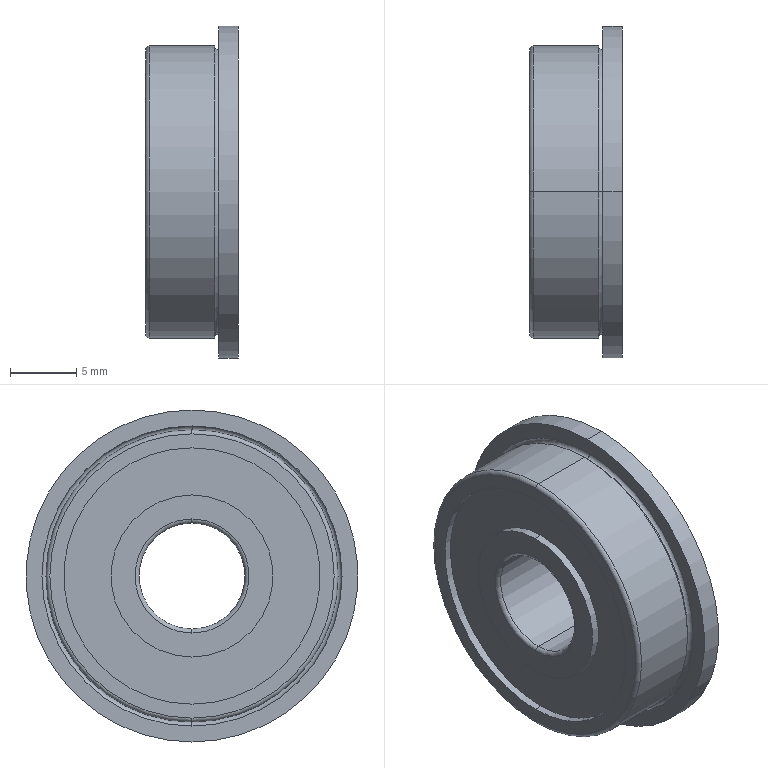Part | SolidWorks | features RefAxis 3, 3DProfileFeature 1, Revolution 1 | 1 solid | 31 faces | box 7 x 25 x 25 mm | volume 2247 mm3 | cylinder 14 | torus 10 | plane 7 | commonest cylinder face diameters 12.2 x4 19.3 x4 8 x2 22 x2 25 x2
STEP:
#1=CARTESIAN_POINT('',(5.2,0.,11.));
#2=VERTEX_POINT('',#1);
#3=CARTESIAN_POINT('',(5.5,0.,10.7));
#4=VERTEX_POINT('',#3);
#5=CARTESIAN_POINT('',(5.5,0.,11.));
#6=DIRECTION('',(0.,-1.,0.));
#7=DIRECTION('',(0.,0.,-1.));
#8=AXIS2_PLACEMENT_3D('',#5,#6,#7);
#9=CIRCLE('',#8,0.3);
#10=EDGE_CURVE('',#2,#4,#9,.T.);
#11=ORIENTED_EDGE('',*,*,#10,.T.);
#12=CARTESIAN_POINT('',(5.5,0.,-10.7));
#13=VERTEX_POINT('',#12);
#14=CARTESIAN_POINT('',(5.5,0.,0.));
#15=DIRECTION('',(-1.,0.,0.));
#16=DIRECTION('',(0.,0.,1.));
#17=AXIS2_PLACEMENT_3D('',#14,#15,#16);
#18=CIRCLE('',#17,10.7);
#19=EDGE_CURVE('',#4,#13,#18,.T.);
#20=ORIENTED_EDGE('',*,*,#19,.T.);
#21=CARTESIAN_POINT('',(5.2,0.,-11.));
#22=VERTEX_POINT('',#21);
#23=CARTESIAN_POINT('',(5.5,0.,-11.));
#24=DIRECTION('',(0.,1.,0.));
#25=DIRECTION('',(0.,0.,1.));
#26=AXIS2_PLACEMENT_3D('',#23,#24,#25);
#27=CIRCLE('',#26,0.3);
#28=EDGE_CURVE('',#22,#13,#27,.T.);
#29=ORIENTED_EDGE('',*,*,#28,.F.);
#30=CARTESIAN_POINT('',(5.2,0.,0.));
#31=DIRECTION('',(-1.,0.,0.));
#32=DIRECTION('',(0.,0.,1.));
#33=AXIS2_PLACEMENT_3D('',#30,#31,#32);
#34=CIRCLE('',#33,11.);
#35=EDGE_CURVE('',#2,#22,#34,.T.);
#36=ORIENTED_EDGE('',*,*,#35,.F.);
#37=EDGE_LOOP('',(#11,#20,#29,#36));
#38=FACE_OUTER_BOUND('',#37,.T.);
#39=CARTESIAN_POINT('',(5.5,0.,0.));
#40=DIRECTION('',(-1.,0.,0.));
#41=DIRECTION('',(0.,0.,1.));
#42=AXIS2_PLACEMENT_3D('',#39,#40,#41);
#43=TOROIDAL_SURFACE('',#42,11.,0.3);
#44=ADVANCED_FACE('',(#38),#43,.F.);
#45=ORIENTED_EDGE('',*,*,#28,.T.);
#46=CARTESIAN_POINT('',(5.5,0.,0.));
#47=DIRECTION('',(-1.,0.,0.));
#48=DIRECTION('',(0.,0.,1.));
#49=AXIS2_PLACEMENT_3D('',#46,#47,#48);
#50=CIRCLE('',#49,10.7);
#51=EDGE_CURVE('',#13,#4,#50,.T.);
#52=ORIENTED_EDGE('',*,*,#51,.T.);
#53=ORIENTED_EDGE('',*,*,#10,.F.);
#54=CARTESIAN_POINT('',(5.2,0.,0.));
#55=DIRECTION('',(-1.,0.,0.));
#56=DIRECTION('',(0.,0.,1.));
#57=AXIS2_PLACEMENT_3D('',#54,#55,#56);
#58=CIRCLE('',#57,11.);
#59=EDGE_CURVE('',#22,#2,#58,.T.);
#60=ORIENTED_EDGE('',*,*,#59,.F.);
#61=EDGE_LOOP('',(#45,#52,#53,#60));
#62=FACE_OUTER_BOUND('',#61,.T.);
#63=CARTESIAN_POINT('',(5.5,0.,0.));
#64=DIRECTION('',(-1.,0.,0.));
#65=DIRECTION('',(0.,0.,1.));
#66=AXIS2_PLACEMENT_3D('',#63,#64,#65);
#67=TOROIDAL_SURFACE('',#66,11.,0.3);
#68=ADVANCED_FACE('',(#62),#67,.F.);
#69=ORIENTED_EDGE('',*,*,#35,.T.);
#70=CARTESIAN_POINT('',(0.3,0.,-11.));
#71=VERTEX_POINT('',#70);
#72=CARTESIAN_POINT('',(22.,0.,-11.));
#73=DIRECTION('',(-1.,0.,0.));
#74=VECTOR('',#73,1000.);
#75=LINE('',#72,#74);
#76=EDGE_CURVE('',#22,#71,#75,.T.);
#77=ORIENTED_EDGE('',*,*,#76,.T.);
#78=CARTESIAN_POINT('',(0.3,0.,11.));
#79=VERTEX_POINT('',#78);
#80=CARTESIAN_POINT('',(0.3,0.,0.));
#81=DIRECTION('',(-1.,0.,0.));
#82=DIRECTION('',(0.,0.,1.));
#83=AXIS2_PLACEMENT_3D('',#80,#81,#82);
#84=CIRCLE('',#83,11.);
#85=EDGE_CURVE('',#79,#71,#84,.T.);
#86=ORIENTED_EDGE('',*,*,#85,.F.);
#87=CARTESIAN_POINT('',(22.,0.,11.));
#88=DIRECTION('',(-1.,0.,0.));
#89=VECTOR('',#88,1000.);
#90=LINE('',#87,#89);
#91=EDGE_CURVE('',#2,#79,#90,.T.);
#92=ORIENTED_EDGE('',*,*,#91,.F.);
#93=EDGE_LOOP('',(#69,#77,#86,#92));
#94=FACE_OUTER_BOUND('',#93,.T.);
#95=CARTESIAN_POINT('',(22.,0.,0.));
#96=DIRECTION('',(-1.,0.,0.));
#97=DIRECTION('',(0.,0.,1.));
#98=AXIS2_PLACEMENT_3D('',#95,#96,#97);
#99=CYLINDRICAL_SURFACE('',#98,11.);
#100=ADVANCED_FACE('',(#94),#99,.T.);
#101=ORIENTED_EDGE('',*,*,#51,.F.);
#102=CARTESIAN_POINT('',(5.5,0.,-11.3));
#103=VERTEX_POINT('',#102);
#104=CARTESIAN_POINT('',(5.5,0.,-11.));
#105=DIRECTION('',(0.,1.,0.));
#106=DIRECTION('',(0.,0.,1.));
#107=AXIS2_PLACEMENT_3D('',#104,#105,#106);
#108=CIRCLE('',#107,0.3);
#109=EDGE_CURVE('',#13,#103,#108,.T.);
#110=ORIENTED_EDGE('',*,*,#109,.T.);
#111=CARTESIAN_POINT('',(5.5,0.,11.3));
#112=VERTEX_POINT('',#111);
#113=CARTESIAN_POINT('',(5.5,0.,0.));
#114=DIRECTION('',(-1.,0.,0.));
#115=DIRECTION('',(0.,0.,1.));
#116=AXIS2_PLACEMENT_3D('',#113,#114,#115);
#117=CIRCLE('',#116,11.3);
#118=EDGE_CURVE('',#103,#112,#117,.T.);
#119=ORIENTED_EDGE('',*,*,#118,.T.);
#120=CARTESIAN_POINT('',(5.5,0.,11.));
#121=DIRECTION('',(0.,-1.,0.));
#122=DIRECTION('',(0.,0.,-1.));
#123=AXIS2_PLACEMENT_3D('',#120,#121,#122);
#124=CIRCLE('',#123,0.3);
#125=EDGE_CURVE('',#4,#112,#124,.T.);
#126=ORIENTED_EDGE('',*,*,#125,.F.);
#127=EDGE_LOOP('',(#101,#110,#119,#126));
#128=FACE_OUTER_BOUND('',#127,.T.);
#129=CARTESIAN_POINT('',(5.5,0.,0.));
#130=DIRECTION('',(-1.,0.,0.));
#131=DIRECTION('',(0.,0.,1.));
#132=AXIS2_PLACEMENT_3D('',#129,#130,#131);
#133=TOROIDAL_SURFACE('',#132,11.,0.3);
#134=ADVANCED_FACE('',(#128),#133,.F.);
#135=CARTESIAN_POINT('',(7.,0.,12.5));
#136=VERTEX_POINT('',#135);
#137=CARTESIAN_POINT('',(7.,0.,-12.5));
#138=VERTEX_POINT('',#137);
#139=CARTESIAN_POINT('',(7.,0.,0.));
#140=DIRECTION('',(-1.,0.,0.));
#141=DIRECTION('',(0.,0.,1.));
#142=AXIS2_PLACEMENT_3D('',#139,#140,#141);
#143=CIRCLE('',#142,12.5);
#144=EDGE_CURVE('',#136,#138,#143,.T.);
#145=ORIENTED_EDGE('',*,*,#144,.T.);
#146=CARTESIAN_POINT('',(5.5,0.,-12.5));
#147=VERTEX_POINT('',#146);
#148=CARTESIAN_POINT('',(22.,0.,-12.5));
#149=DIRECTION('',(-1.,0.,0.));
#150=VECTOR('',#149,1000.);
#151=LINE('',#148,#150);
#152=EDGE_CURVE('',#138,#147,#151,.T.);
#153=ORIENTED_EDGE('',*,*,#152,.T.);
#154=CARTESIAN_POINT('',(5.5,0.,12.5));
#155=VERTEX_POINT('',#154);
#156=CARTESIAN_POINT('',(5.5,0.,0.));
#157=DIRECTION('',(-1.,0.,0.));
#158=DIRECTION('',(0.,0.,1.));
#159=AXIS2_PLACEMENT_3D('',#156,#157,#158);
#160=CIRCLE('',#159,12.5);
#161=EDGE_CURVE('',#155,#147,#160,.T.);
#162=ORIENTED_EDGE('',*,*,#161,.F.);
#163=CARTESIAN_POINT('',(22.,0.,12.5));
#164=DIRECTION('',(-1.,0.,0.));
#165=VECTOR('',#164,1000.);
#166=LINE('',#163,#165);
#167=EDGE_CURVE('',#136,#155,#166,.T.);
#168=ORIENTED_EDGE('',*,*,#167,.F.);
#169=EDGE_LOOP('',(#145,#153,#162,#168));
#170=FACE_OUTER_BOUND('',#169,.T.);
#171=CARTESIAN_POINT('',(22.,0.,0.));
#172=DIRECTION('',(-1.,0.,0.));
#173=DIRECTION('',(0.,0.,1.));
#174=AXIS2_PLACEMENT_3D('',#171,#172,#173);
#175=CYLINDRICAL_SURFACE('',#174,12.5);
#176=ADVANCED_FACE('',(#170),#175,.T.);
#177=CARTESIAN_POINT('',(7.,0.,-9.65));
#178=VERTEX_POINT('',#177);
#179=CARTESIAN_POINT('',(7.,0.,9.65));
#180=VERTEX_POINT('',#179);
#181=CARTESIAN_POINT('',(7.,0.,0.));
#182=DIRECTION('',(-1.,0.,0.));
#183=DIRECTION('',(0.,0.,1.));
#184=AXIS2_PLACEMENT_3D('',#181,#182,#183);
#185=CIRCLE('',#184,9.65);
#186=EDGE_CURVE('',#178,#180,#185,.T.);
#187=ORIENTED_EDGE('',*,*,#186,.F.);
#188=CARTESIAN_POINT('',(6.4,0.,-9.65));
#189=VERTEX_POINT('',#188);
#190=CARTESIAN_POINT('',(22.,0.,-9.65));
#191=DIRECTION('',(-1.,0.,0.));
#192=VECTOR('',#191,1000.);
#193=LINE('',#190,#192);
#194=EDGE_CURVE('',#178,#189,#193,.T.);
#195=ORIENTED_EDGE('',*,*,#194,.T.);
#196=CARTESIAN_POINT('',(6.4,0.,9.65));
#197=VERTEX_POINT('',#196);
#198=CARTESIAN_POINT('',(6.4,0.,0.));
#199=DIRECTION('',(-1.,0.,0.));
#200=DIRECTION('',(0.,0.,1.));
#201=AXIS2_PLACEMENT_3D('',#198,#199,#200);
#202=CIRCLE('',#201,9.65);
#203=EDGE_CURVE('',#189,#197,#202,.T.);
#204=ORIENTED_EDGE('',*,*,#203,.T.);
#205=CARTESIAN_POINT('',(22.,0.,9.65));
#206=DIRECTION('',(-1.,0.,0.));
#207=VECTOR('',#206,1000.);
#208=LINE('',#205,#207);
#209=EDGE_CURVE('',#180,#197,#208,.T.);
#210=ORIENTED_EDGE('',*,*,#209,.F.);
#211=EDGE_LOOP('',(#187,#195,#204,#210));
#212=FACE_OUTER_BOUND('',#211,.T.);
#213=CARTESIAN_POINT('',(22.,0.,0.));
#214=DIRECTION('',(-1.,0.,0.));
#215=DIRECTION('',(0.,0.,1.));
#216=AXIS2_PLACEMENT_3D('',#213,#214,#215);
#217=CYLINDRICAL_SURFACE('',#216,9.65);
#218=ADVANCED_FACE('',(#212),#217,.F.);
#219=CARTESIAN_POINT('',(7.,0.,6.1));
#220=VERTEX_POINT('',#219);
#221=CARTESIAN_POINT('',(7.,0.,-6.1));
#222=VERTEX_POINT('',#221);
#223=CARTESIAN_POINT('',(7.,0.,0.));
#224=DIRECTION('',(-1.,0.,0.));
#225=DIRECTION('',(0.,0.,1.));
#226=AXIS2_PLACEMENT_3D('',#223,#224,#225);
#227=CIRCLE('',#226,6.1);
#228=EDGE_CURVE('',#220,#222,#227,.T.);
#229=ORIENTED_EDGE('',*,*,#228,.T.);
#230=CARTESIAN_POINT('',(6.4,0.,-6.1));
#231=VERTEX_POINT('',#230);
#232=CARTESIAN_POINT('',(22.,0.,-6.1));
#233=DIRECTION('',(-1.,0.,0.));
#234=VECTOR('',#233,1000.);
#235=LINE('',#232,#234);
#236=EDGE_CURVE('',#222,#231,#235,.T.);
#237=ORIENTED_EDGE('',*,*,#236,.T.);
#238=CARTESIAN_POINT('',(6.4,0.,6.1));
#239=VERTEX_POINT('',#238);
#240=CARTESIAN_POINT('',(6.4,0.,0.));
#241=DIRECTION('',(-1.,0.,0.));
#242=DIRECTION('',(0.,0.,1.));
#243=AXIS2_PLACEMENT_3D('',#240,#241,#242);
#244=CIRCLE('',#243,6.1);
#245=EDGE_CURVE('',#239,#231,#244,.T.);
#246=ORIENTED_EDGE('',*,*,#245,.F.);
#247=CARTESIAN_POINT('',(22.,0.,6.1));
#248=DIRECTION('',(-1.,0.,0.));
#249=VECTOR('',#248,1000.);
#250=LINE('',#247,#249);
#251=EDGE_CURVE('',#220,#239,#250,.T.);
#252=ORIENTED_EDGE('',*,*,#251,.F.);
#253=EDGE_LOOP('',(#229,#237,#246,#252));
#254=FACE_OUTER_BOUND('',#253,.T.);
#255=CARTESIAN_POINT('',(22.,0.,0.));
#256=DIRECTION('',(-1.,0.,0.));
#257=DIRECTION('',(0.,0.,1.));
#258=AXIS2_PLACEMENT_3D('',#255,#256,#257);
#259=CYLINDRICAL_SURFACE('',#258,6.1);
#260=ADVANCED_FACE('',(#254),#259,.T.);
#261=CARTESIAN_POINT('',(6.7,0.,4.));
#262=VERTEX_POINT('',#261);
#263=CARTESIAN_POINT('',(6.7,0.,-4.));
#264=VERTEX_POINT('',#263);
#265=CARTESIAN_POINT('',(6.7,0.,0.));
#266=DIRECTION('',(-1.,0.,0.));
#267=DIRECTION('',(0.,0.,1.));
#268=AXIS2_PLACEMENT_3D('',#265,#266,#267);
#269=CIRCLE('',#268,4.);
#270=EDGE_CURVE('',#262,#264,#269,.T.);
#271=ORIENTED_EDGE('',*,*,#270,.T.);
#272=CARTESIAN_POINT('',(7.,0.,-4.3));
#273=VERTEX_POINT('',#272);
#274=CARTESIAN_POINT('',(6.7,0.,-4.3));
#275=DIRECTION('',(0.,1.,0.));
#276=DIRECTION('',(0.,0.,1.));
#277=AXIS2_PLACEMENT_3D('',#274,#275,#276);
#278=CIRCLE('',#277,0.3);
#279=EDGE_CURVE('',#264,#273,#278,.T.);
#280=ORIENTED_EDGE('',*,*,#279,.T.);
#281=CARTESIAN_POINT('',(7.,0.,4.3));
#282=VERTEX_POINT('',#281);
#283=CARTESIAN_POINT('',(7.,0.,0.));
#284=DIRECTION('',(-1.,0.,0.));
#285=DIRECTION('',(0.,0.,1.));
#286=AXIS2_PLACEMENT_3D('',#283,#284,#285);
#287=CIRCLE('',#286,4.3);
#288=EDGE_CURVE('',#282,#273,#287,.T.);
#289=ORIENTED_EDGE('',*,*,#288,.F.);
#290=CARTESIAN_POINT('',(6.7,0.,4.3));
#291=DIRECTION('',(0.,-1.,0.));
#292=DIRECTION('',(0.,0.,-1.));
#293=AXIS2_PLACEMENT_3D('',#290,#291,#292);
#294=CIRCLE('',#293,0.3);
#295=EDGE_CURVE('',#262,#282,#294,.T.);
#296=ORIENTED_EDGE('',*,*,#295,.F.);
#297=EDGE_LOOP('',(#271,#280,#289,#296));
#298=FACE_OUTER_BOUND('',#297,.T.);
#299=CARTESIAN_POINT('',(6.7,0.,0.));
#300=DIRECTION('',(-1.,0.,0.));
#301=DIRECTION('',(0.,0.,1.));
#302=AXIS2_PLACEMENT_3D('',#299,#300,#301);
#303=TOROIDAL_SURFACE('',#302,4.3,0.3);
#304=ADVANCED_FACE('',(#298),#303,.T.);
#305=CARTESIAN_POINT('',(6.7,0.,0.));
#306=DIRECTION('',(-1.,0.,0.));
#307=DIRECTION('',(0.,0.,1.));
#308=AXIS2_PLACEMENT_3D('',#305,#306,#307);
#309=CIRCLE('',#308,4.);
#310=EDGE_CURVE('',#264,#262,#309,.T.);
#311=ORIENTED_EDGE('',*,*,#310,.F.);
#312=CARTESIAN_POINT('',(0.3,0.,-4.));
#313=VERTEX_POINT('',#312);
#314=CARTESIAN_POINT('',(22.,0.,-4.));
#315=DIRECTION('',(-1.,0.,0.));
#316=VECTOR('',#315,1000.);
#317=LINE('',#314,#316);
#318=EDGE_CURVE('',#264,#313,#317,.T.);
#319=ORIENTED_EDGE('',*,*,#318,.T.);
#320=CARTESIAN_POINT('',(0.3,0.,4.));
#321=VERTEX_POINT('',#320);
#322=CARTESIAN_POINT('',(0.3,0.,0.));
#323=DIRECTION('',(-1.,0.,0.));
#324=DIRECTION('',(0.,0.,1.));
#325=AXIS2_PLACEMENT_3D('',#322,#323,#324);
#326=CIRCLE('',#325,4.);
#327=EDGE_CURVE('',#313,#321,#326,.T.);
#328=ORIENTED_EDGE('',*,*,#327,.T.);
#329=CARTESIAN_POINT('',(22.,0.,4.));
#330=DIRECTION('',(-1.,0.,0.));
#331=VECTOR('',#330,1000.);
#332=LINE('',#329,#331);
#333=EDGE_CURVE('',#262,#321,#332,.T.);
#334=ORIENTED_EDGE('',*,*,#333,.F.);
#335=EDGE_LOOP('',(#311,#319,#328,#334));
#336=FACE_OUTER_BOUND('',#335,.T.);
#337=CARTESIAN_POINT('',(22.,0.,0.));
#338=DIRECTION('',(-1.,0.,0.));
#339=DIRECTION('',(0.,0.,1.));
#340=AXIS2_PLACEMENT_3D('',#337,#338,#339);
#341=CYLINDRICAL_SURFACE('',#340,4.);
#342=ADVANCED_FACE('',(#336),#341,.F.);
#343=CARTESIAN_POINT('',(0.,0.,4.3));
#344=VERTEX_POINT('',#343);
#345=CARTESIAN_POINT('',(0.,0.,-4.3));
#346=VERTEX_POINT('',#345);
#347=CARTESIAN_POINT('',(0.,0.,0.));
#348=DIRECTION('',(-1.,0.,0.));
#349=DIRECTION('',(0.,0.,1.));
#350=AXIS2_PLACEMENT_3D('',#347,#348,#349);
#351=CIRCLE('',#350,4.3);
#352=EDGE_CURVE('',#344,#346,#351,.T.);
#353=ORIENTED_EDGE('',*,*,#352,.T.);
#354=CARTESIAN_POINT('',(0.3,0.,-4.3));
#355=DIRECTION('',(0.,1.,0.));
#356=DIRECTION('',(0.,0.,1.));
#357=AXIS2_PLACEMENT_3D('',#354,#355,#356);
#358=CIRCLE('',#357,0.3);
#359=EDGE_CURVE('',#346,#313,#358,.T.);
#360=ORIENTED_EDGE('',*,*,#359,.T.);
#361=CARTESIAN_POINT('',(0.3,0.,0.));
#362=DIRECTION('',(-1.,0.,0.));
#363=DIRECTION('',(0.,0.,1.));
#364=AXIS2_PLACEMENT_3D('',#361,#362,#363);
#365=CIRCLE('',#364,4.);
#366=EDGE_CURVE('',#321,#313,#365,.T.);
#367=ORIENTED_EDGE('',*,*,#366,.F.);
#368=CARTESIAN_POINT('',(0.3,0.,4.3));
#369=DIRECTION('',(0.,-1.,0.));
#370=DIRECTION('',(0.,0.,-1.));
#371=AXIS2_PLACEMENT_3D('',#368,#369,#370);
#372=CIRCLE('',#371,0.3);
#373=EDGE_CURVE('',#344,#321,#372,.T.);
#374=ORIENTED_EDGE('',*,*,#373,.F.);
#375=EDGE_LOOP('',(#353,#360,#367,#374));
#376=FACE_OUTER_BOUND('',#375,.T.);
#377=CARTESIAN_POINT('',(0.3,0.,0.));
#378=DIRECTION('',(-1.,0.,0.));
#379=DIRECTION('',(0.,0.,1.));
#380=AXIS2_PLACEMENT_3D('',#377,#378,#379);
#381=TOROIDAL_SURFACE('',#380,4.3,0.3);
#382=ADVANCED_FACE('',(#376),#381,.T.);
#383=CARTESIAN_POINT('',(0.6,0.,6.1));
#384=VERTEX_POINT('',#383);
#385=CARTESIAN_POINT('',(0.6,0.,-6.1));
#386=VERTEX_POINT('',#385);
#387=CARTESIAN_POINT('',(0.6,0.,0.));
#388=DIRECTION('',(-1.,0.,0.));
#389=DIRECTION('',(0.,0.,1.));
#390=AXIS2_PLACEMENT_3D('',#387,#388,#389);
#391=CIRCLE('',#390,6.1);
#392=EDGE_CURVE('',#384,#386,#391,.T.);
#393=ORIENTED_EDGE('',*,*,#392,.T.);
#394=CARTESIAN_POINT('',(0.,0.,-6.1));
#395=VERTEX_POINT('',#394);
#396=CARTESIAN_POINT('',(22.,0.,-6.1));
#397=DIRECTION('',(-1.,0.,0.));
#398=VECTOR('',#397,1000.);
#399=LINE('',#396,#398);
#400=EDGE_CURVE('',#386,#395,#399,.T.);
#401=ORIENTED_EDGE('',*,*,#400,.T.);
#402=CARTESIAN_POINT('',(0.,0.,6.1));
#403=VERTEX_POINT('',#402);
#404=CARTESIAN_POINT('',(0.,0.,0.));
#405=DIRECTION('',(-1.,0.,0.));
#406=DIRECTION('',(0.,0.,1.));
#407=AXIS2_PLACEMENT_3D('',#404,#405,#406);
#408=CIRCLE('',#407,6.1);
#409=EDGE_CURVE('',#403,#395,#408,.T.);
#410=ORIENTED_EDGE('',*,*,#409,.F.);
#411=CARTESIAN_POINT('',(22.,0.,6.1));
#412=DIRECTION('',(-1.,0.,0.));
#413=VECTOR('',#412,1000.);
#414=LINE('',#411,#413);
#415=EDGE_CURVE('',#384,#403,#414,.T.);
#416=ORIENTED_EDGE('',*,*,#415,.F.);
#417=EDGE_LOOP('',(#393,#401,#410,#416));
#418=FACE_OUTER_BOUND('',#417,.T.);
#419=CARTESIAN_POINT('',(22.,0.,0.));
#420=DIRECTION('',(-1.,0.,0.));
#421=DIRECTION('',(0.,0.,1.));
#422=AXIS2_PLACEMENT_3D('',#419,#420,#421);
#423=CYLINDRICAL_SURFACE('',#422,6.1);
#424=ADVANCED_FACE('',(#418),#423,.T.);
#425=CARTESIAN_POINT('',(0.6,0.,-9.65));
#426=VERTEX_POINT('',#425);
#427=CARTESIAN_POINT('',(0.6,0.,9.65));
#428=VERTEX_POINT('',#427);
#429=CARTESIAN_POINT('',(0.6,0.,0.));
#430=DIRECTION('',(-1.,0.,0.));
#431=DIRECTION('',(0.,0.,1.));
#432=AXIS2_PLACEMENT_3D('',#429,#430,#431);
#433=CIRCLE('',#432,9.65);
#434=EDGE_CURVE('',#426,#428,#433,.T.);
#435=ORIENTED_EDGE('',*,*,#434,.F.);
#436=CARTESIAN_POINT('',(0.,0.,-9.65));
#437=VERTEX_POINT('',#436);
#438=CARTESIAN_POINT('',(22.,0.,-9.65));
#439=DIRECTION('',(-1.,0.,0.));
#440=VECTOR('',#439,1000.);
#441=LINE('',#438,#440);
#442=EDGE_CURVE('',#426,#437,#441,.T.);
#443=ORIENTED_EDGE('',*,*,#442,.T.);
#444=CARTESIAN_POINT('',(0.,0.,9.65));
#445=VERTEX_POINT('',#444);
#446=CARTESIAN_POINT('',(0.,0.,0.));
#447=DIRECTION('',(-1.,0.,0.));
#448=DIRECTION('',(0.,0.,1.));
#449=AXIS2_PLACEMENT_3D('',#446,#447,#448);
#450=CIRCLE('',#449,9.65);
#451=EDGE_CURVE('',#437,#445,#450,.T.);
#452=ORIENTED_EDGE('',*,*,#451,.T.);
#453=CARTESIAN_POINT('',(22.,0.,9.65));
#454=DIRECTION('',(-1.,0.,0.));
#455=VECTOR('',#454,1000.);
#456=LINE('',#453,#455);
#457=EDGE_CURVE('',#428,#445,#456,.T.);
#458=ORIENTED_EDGE('',*,*,#457,.F.);
#459=EDGE_LOOP('',(#435,#443,#452,#458));
#460=FACE_OUTER_BOUND('',#459,.T.);
#461=CARTESIAN_POINT('',(22.,0.,0.));
#462=DIRECTION('',(-1.,0.,0.));
#463=DIRECTION('',(0.,0.,1.));
#464=AXIS2_PLACEMENT_3D('',#461,#462,#463);
#465=CYLINDRICAL_SURFACE('',#464,9.65);
#466=ADVANCED_FACE('',(#460),#465,.F.);
#467=ORIENTED_EDGE('',*,*,#85,.T.);
#468=CARTESIAN_POINT('',(0.,0.,-10.7));
#469=VERTEX_POINT('',#468);
#470=CARTESIAN_POINT('',(0.3,0.,-10.7));
#471=DIRECTION('',(0.,1.,0.));
#472=DIRECTION('',(0.,0.,1.));
#473=AXIS2_PLACEMENT_3D('',#470,#471,#472);
#474=CIRCLE('',#473,0.3);
#475=EDGE_CURVE('',#71,#469,#474,.T.);
#476=ORIENTED_EDGE('',*,*,#475,.T.);
#477=CARTESIAN_POINT('',(0.,0.,10.7));
#478=VERTEX_POINT('',#477);
#479=CARTESIAN_POINT('',(0.,0.,0.));
#480=DIRECTION('',(-1.,0.,0.));
#481=DIRECTION('',(0.,0.,1.));
#482=AXIS2_PLACEMENT_3D('',#479,#480,#481);
#483=CIRCLE('',#482,10.7);
#484=EDGE_CURVE('',#478,#469,#483,.T.);
#485=ORIENTED_EDGE('',*,*,#484,.F.);
#486=CARTESIAN_POINT('',(0.3,0.,10.7));
#487=DIRECTION('',(0.,-1.,0.));
#488=DIRECTION('',(0.,0.,-1.));
#489=AXIS2_PLACEMENT_3D('',#486,#487,#488);
#490=CIRCLE('',#489,0.3);
#491=EDGE_CURVE('',#79,#478,#490,.T.);
#492=ORIENTED_EDGE('',*,*,#491,.F.);
#493=EDGE_LOOP('',(#467,#476,#485,#492));
#494=FACE_OUTER_BOUND('',#493,.T.);
#495=CARTESIAN_POINT('',(0.3,0.,0.));
#496=DIRECTION('',(-1.,0.,0.));
#497=DIRECTION('',(0.,0.,1.));
#498=AXIS2_PLACEMENT_3D('',#495,#496,#497);
#499=TOROIDAL_SURFACE('',#498,10.7,0.3);
#500=ADVANCED_FACE('',(#494),#499,.T.);
#501=ORIENTED_EDGE('',*,*,#475,.F.);
#502=CARTESIAN_POINT('',(0.3,0.,0.));
#503=DIRECTION('',(-1.,0.,0.));
#504=DIRECTION('',(0.,0.,1.));
#505=AXIS2_PLACEMENT_3D('',#502,#503,#504);
#506=CIRCLE('',#505,11.);
#507=EDGE_CURVE('',#71,#79,#506,.T.);
#508=ORIENTED_EDGE('',*,*,#507,.T.);
#509=ORIENTED_EDGE('',*,*,#491,.T.);
#510=CARTESIAN_POINT('',(0.,0.,0.));
#511=DIRECTION('',(-1.,0.,0.));
#512=DIRECTION('',(0.,0.,1.));
#513=AXIS2_PLACEMENT_3D('',#510,#511,#512);
#514=CIRCLE('',#513,10.7);
#515=EDGE_CURVE('',#469,#478,#514,.T.);
#516=ORIENTED_EDGE('',*,*,#515,.F.);
#517=EDGE_LOOP('',(#501,#508,#509,#516));
#518=FACE_OUTER_BOUND('',#517,.T.);
#519=CARTESIAN_POINT('',(0.3,0.,0.));
#520=DIRECTION('',(-1.,0.,0.));
#521=DIRECTION('',(0.,0.,1.));
#522=AXIS2_PLACEMENT_3D('',#519,#520,#521);
#523=TOROIDAL_SURFACE('',#522,10.7,0.3);
#524=ADVANCED_FACE('',(#518),#523,.T.);
#525=CARTESIAN_POINT('',(0.,0.,0.));
#526=DIRECTION('',(-1.,0.,0.));
#527=DIRECTION('',(0.,0.,1.));
#528=AXIS2_PLACEMENT_3D('',#525,#526,#527);
#529=CIRCLE('',#528,9.65);
#530=EDGE_CURVE('',#445,#437,#529,.T.);
#531=ORIENTED_EDGE('',*,*,#530,.F.);
#532=ORIENTED_EDGE('',*,*,#451,.F.);
#533=EDGE_LOOP('',(#531,#532));
#534=FACE_BOUND('',#533,.T.);
#535=ORIENTED_EDGE('',*,*,#484,.T.);
#536=ORIENTED_EDGE('',*,*,#515,.T.);
#537=EDGE_LOOP('',(#535,#536));
#538=FACE_OUTER_BOUND('',#537,.T.);
#539=CARTESIAN_POINT('',(0.,10.7,0.));
#540=DIRECTION('',(1.,0.,0.));
#541=DIRECTION('',(0.,0.,-1.));
#542=AXIS2_PLACEMENT_3D('',#539,#540,#541);
#543=PLANE('',#542);
#544=ADVANCED_FACE('',(#534,#538),#543,.F.);
#545=ORIENTED_EDGE('',*,*,#442,.F.);
#546=CARTESIAN_POINT('',(0.6,0.,0.));
#547=DIRECTION('',(-1.,0.,0.));
#548=DIRECTION('',(0.,0.,1.));
#549=AXIS2_PLACEMENT_3D('',#546,#547,#548);
#550=CIRCLE('',#549,9.65);
#551=EDGE_CURVE('',#428,#426,#550,.T.);
#552=ORIENTED_EDGE('',*,*,#551,.F.);
#553=ORIENTED_EDGE('',*,*,#457,.T.);
#554=ORIENTED_EDGE('',*,*,#530,.T.);
#555=EDGE_LOOP('',(#545,#552,#553,#554));
#556=FACE_OUTER_BOUND('',#555,.T.);
#557=CARTESIAN_POINT('',(22.,0.,0.));
#558=DIRECTION('',(-1.,0.,0.));
#559=DIRECTION('',(0.,0.,1.));
#560=AXIS2_PLACEMENT_3D('',#557,#558,#559);
#561=CYLINDRICAL_SURFACE('',#560,9.65);
#562=ADVANCED_FACE('',(#556),#561,.F.);
#563=ORIENTED_EDGE('',*,*,#392,.F.);
#564=CARTESIAN_POINT('',(0.6,0.,0.));
#565=DIRECTION('',(-1.,0.,0.));
#566=DIRECTION('',(0.,0.,1.));
#567=AXIS2_PLACEMENT_3D('',#564,#565,#566);
#568=CIRCLE('',#567,6.1);
#569=EDGE_CURVE('',#386,#384,#568,.T.);
#570=ORIENTED_EDGE('',*,*,#569,.F.);
#571=EDGE_LOOP('',(#563,#570));
#572=FACE_BOUND('',#571,.T.);
#573=ORIENTED_EDGE('',*,*,#551,.T.);
#574=ORIENTED_EDGE('',*,*,#434,.T.);
#575=EDGE_LOOP('',(#573,#574));
#576=FACE_OUTER_BOUND('',#575,.T.);
#577=CARTESIAN_POINT('',(0.6,9.65,0.));
#578=DIRECTION('',(1.,0.,0.));
#579=DIRECTION('',(0.,0.,-1.));
#580=AXIS2_PLACEMENT_3D('',#577,#578,#579);
#581=PLANE('',#580);
#582=ADVANCED_FACE('',(#572,#576),#581,.F.);
#583=ORIENTED_EDGE('',*,*,#400,.F.);
#584=ORIENTED_EDGE('',*,*,#569,.T.);
#585=ORIENTED_EDGE('',*,*,#415,.T.);
#586=CARTESIAN_POINT('',(0.,0.,0.));
#587=DIRECTION('',(-1.,0.,0.));
#588=DIRECTION('',(0.,0.,1.));
#589=AXIS2_PLACEMENT_3D('',#586,#587,#588);
#590=CIRCLE('',#589,6.1);
#591=EDGE_CURVE('',#395,#403,#590,.T.);
#592=ORIENTED_EDGE('',*,*,#591,.F.);
#593=EDGE_LOOP('',(#583,#584,#585,#592));
#594=FACE_OUTER_BOUND('',#593,.T.);
#595=CARTESIAN_POINT('',(22.,0.,0.));
#596=DIRECTION('',(-1.,0.,0.));
#597=DIRECTION('',(0.,0.,1.));
#598=AXIS2_PLACEMENT_3D('',#595,#596,#597);
#599=CYLINDRICAL_SURFACE('',#598,6.1);
#600=ADVANCED_FACE('',(#594),#599,.T.);
#601=ORIENTED_EDGE('',*,*,#352,.F.);
#602=CARTESIAN_POINT('',(0.,0.,0.));
#603=DIRECTION('',(-1.,0.,0.));
#604=DIRECTION('',(0.,0.,1.));
#605=AXIS2_PLACEMENT_3D('',#602,#603,#604);
#606=CIRCLE('',#605,4.3);
#607=EDGE_CURVE('',#346,#344,#606,.T.);
#608=ORIENTED_EDGE('',*,*,#607,.F.);
#609=EDGE_LOOP('',(#601,#608));
#610=FACE_BOUND('',#609,.T.);
#611=ORIENTED_EDGE('',*,*,#409,.T.);
#612=ORIENTED_EDGE('',*,*,#591,.T.);
#613=EDGE_LOOP('',(#611,#612));
#614=FACE_OUTER_BOUND('',#613,.T.);
#615=CARTESIAN_POINT('',(0.,6.1,0.));
#616=DIRECTION('',(1.,0.,0.));
#617=DIRECTION('',(0.,0.,-1.));
#618=AXIS2_PLACEMENT_3D('',#615,#616,#617);
#619=PLANE('',#618);
#620=ADVANCED_FACE('',(#610,#614),#619,.F.);
#621=ORIENTED_EDGE('',*,*,#359,.F.);
#622=ORIENTED_EDGE('',*,*,#607,.T.);
#623=ORIENTED_EDGE('',*,*,#373,.T.);
#624=ORIENTED_EDGE('',*,*,#327,.F.);
#625=EDGE_LOOP('',(#621,#622,#623,#624));
#626=FACE_OUTER_BOUND('',#625,.T.);
#627=CARTESIAN_POINT('',(0.3,0.,0.));
#628=DIRECTION('',(-1.,0.,0.));
#629=DIRECTION('',(0.,0.,1.));
#630=AXIS2_PLACEMENT_3D('',#627,#628,#629);
#631=TOROIDAL_SURFACE('',#630,4.3,0.3);
#632=ADVANCED_FACE('',(#626),#631,.T.);
#633=ORIENTED_EDGE('',*,*,#318,.F.);
#634=ORIENTED_EDGE('',*,*,#270,.F.);
#635=ORIENTED_EDGE('',*,*,#333,.T.);
#636=ORIENTED_EDGE('',*,*,#366,.T.);
#637=EDGE_LOOP('',(#633,#634,#635,#636));
#638=FACE_OUTER_BOUND('',#637,.T.);
#639=CARTESIAN_POINT('',(22.,0.,0.));
#640=DIRECTION('',(-1.,0.,0.));
#641=DIRECTION('',(0.,0.,1.));
#642=AXIS2_PLACEMENT_3D('',#639,#640,#641);
#643=CYLINDRICAL_SURFACE('',#642,4.);
#644=ADVANCED_FACE('',(#638),#643,.F.);
#645=ORIENTED_EDGE('',*,*,#279,.F.);
#646=ORIENTED_EDGE('',*,*,#310,.T.);
#647=ORIENTED_EDGE('',*,*,#295,.T.);
#648=CARTESIAN_POINT('',(7.,0.,0.));
#649=DIRECTION('',(-1.,0.,0.));
#650=DIRECTION('',(0.,0.,1.));
#651=AXIS2_PLACEMENT_3D('',#648,#649,#650);
#652=CIRCLE('',#651,4.3);
#653=EDGE_CURVE('',#273,#282,#652,.T.);
#654=ORIENTED_EDGE('',*,*,#653,.F.);
#655=EDGE_LOOP('',(#645,#646,#647,#654));
#656=FACE_OUTER_BOUND('',#655,.T.);
#657=CARTESIAN_POINT('',(6.7,0.,0.));
#658=DIRECTION('',(-1.,0.,0.));
#659=DIRECTION('',(0.,0.,1.));
#660=AXIS2_PLACEMENT_3D('',#657,#658,#659);
#661=TOROIDAL_SURFACE('',#660,4.3,0.3);
#662=ADVANCED_FACE('',(#656),#661,.T.);
#663=ORIENTED_EDGE('',*,*,#228,.F.);
#664=CARTESIAN_POINT('',(7.,0.,0.));
#665=DIRECTION('',(-1.,0.,0.));
#666=DIRECTION('',(0.,0.,1.));
#667=AXIS2_PLACEMENT_3D('',#664,#665,#666);
#668=CIRCLE('',#667,6.1);
#669=EDGE_CURVE('',#222,#220,#668,.T.);
#670=ORIENTED_EDGE('',*,*,#669,.F.);
#671=EDGE_LOOP('',(#663,#670));
#672=FACE_OUTER_BOUND('',#671,.T.);
#673=ORIENTED_EDGE('',*,*,#288,.T.);
#674=ORIENTED_EDGE('',*,*,#653,.T.);
#675=EDGE_LOOP('',(#673,#674));
#676=FACE_BOUND('',#675,.T.);
#677=CARTESIAN_POINT('',(7.,4.3,0.));
#678=DIRECTION('',(-1.,0.,0.));
#679=DIRECTION('',(0.,0.,1.));
#680=AXIS2_PLACEMENT_3D('',#677,#678,#679);
#681=PLANE('',#680);
#682=ADVANCED_FACE('',(#672,#676),#681,.F.);
#683=ORIENTED_EDGE('',*,*,#236,.F.);
#684=ORIENTED_EDGE('',*,*,#669,.T.);
#685=ORIENTED_EDGE('',*,*,#251,.T.);
#686=CARTESIAN_POINT('',(6.4,0.,0.));
#687=DIRECTION('',(-1.,0.,0.));
#688=DIRECTION('',(0.,0.,1.));
#689=AXIS2_PLACEMENT_3D('',#686,#687,#688);
#690=CIRCLE('',#689,6.1);
#691=EDGE_CURVE('',#231,#239,#690,.T.);
#692=ORIENTED_EDGE('',*,*,#691,.F.);
#693=EDGE_LOOP('',(#683,#684,#685,#692));
#694=FACE_OUTER_BOUND('',#693,.T.);
#695=CARTESIAN_POINT('',(22.,0.,0.));
#696=DIRECTION('',(-1.,0.,0.));
#697=DIRECTION('',(0.,0.,1.));
#698=AXIS2_PLACEMENT_3D('',#695,#696,#697);
#699=CYLINDRICAL_SURFACE('',#698,6.1);
#700=ADVANCED_FACE('',(#694),#699,.T.);
#701=CARTESIAN_POINT('',(6.4,0.,0.));
#702=DIRECTION('',(-1.,0.,0.));
#703=DIRECTION('',(0.,0.,1.));
#704=AXIS2_PLACEMENT_3D('',#701,#702,#703);
#705=CIRCLE('',#704,9.65);
#706=EDGE_CURVE('',#197,#189,#705,.T.);
#707=ORIENTED_EDGE('',*,*,#706,.F.);
#708=ORIENTED_EDGE('',*,*,#203,.F.);
#709=EDGE_LOOP('',(#707,#708));
#710=FACE_OUTER_BOUND('',#709,.T.);
#711=ORIENTED_EDGE('',*,*,#245,.T.);
#712=ORIENTED_EDGE('',*,*,#691,.T.);
#713=EDGE_LOOP('',(#711,#712));
#714=FACE_BOUND('',#713,.T.);
#715=CARTESIAN_POINT('',(6.4,6.1,0.));
#716=DIRECTION('',(-1.,0.,0.));
#717=DIRECTION('',(0.,0.,1.));
#718=AXIS2_PLACEMENT_3D('',#715,#716,#717);
#719=PLANE('',#718);
#720=ADVANCED_FACE('',(#710,#714),#719,.F.);
#721=ORIENTED_EDGE('',*,*,#194,.F.);
#722=CARTESIAN_POINT('',(7.,0.,0.));
#723=DIRECTION('',(-1.,0.,0.));
#724=DIRECTION('',(0.,0.,1.));
#725=AXIS2_PLACEMENT_3D('',#722,#723,#724);
#726=CIRCLE('',#725,9.65);
#727=EDGE_CURVE('',#180,#178,#726,.T.);
#728=ORIENTED_EDGE('',*,*,#727,.F.);
#729=ORIENTED_EDGE('',*,*,#209,.T.);
#730=ORIENTED_EDGE('',*,*,#706,.T.);
#731=EDGE_LOOP('',(#721,#728,#729,#730));
#732=FACE_OUTER_BOUND('',#731,.T.);
#733=CARTESIAN_POINT('',(22.,0.,0.));
#734=DIRECTION('',(-1.,0.,0.));
#735=DIRECTION('',(0.,0.,1.));
#736=AXIS2_PLACEMENT_3D('',#733,#734,#735);
#737=CYLINDRICAL_SURFACE('',#736,9.65);
#738=ADVANCED_FACE('',(#732),#737,.F.);
#739=ORIENTED_EDGE('',*,*,#144,.F.);
#740=CARTESIAN_POINT('',(7.,0.,0.));
#741=DIRECTION('',(-1.,0.,0.));
#742=DIRECTION('',(0.,0.,1.));
#743=AXIS2_PLACEMENT_3D('',#740,#741,#742);
#744=CIRCLE('',#743,12.5);
#745=EDGE_CURVE('',#138,#136,#744,.T.);
#746=ORIENTED_EDGE('',*,*,#745,.F.);
#747=EDGE_LOOP('',(#739,#746));
#748=FACE_OUTER_BOUND('',#747,.T.);
#749=ORIENTED_EDGE('',*,*,#727,.T.);
#750=ORIENTED_EDGE('',*,*,#186,.T.);
#751=EDGE_LOOP('',(#749,#750));
#752=FACE_BOUND('',#751,.T.);
#753=CARTESIAN_POINT('',(7.,9.65,0.));
#754=DIRECTION('',(-1.,0.,0.));
#755=DIRECTION('',(0.,0.,1.));
#756=AXIS2_PLACEMENT_3D('',#753,#754,#755);
#757=PLANE('',#756);
#758=ADVANCED_FACE('',(#748,#752),#757,.F.);
#759=ORIENTED_EDGE('',*,*,#152,.F.);
#760=ORIENTED_EDGE('',*,*,#745,.T.);
#761=ORIENTED_EDGE('',*,*,#167,.T.);
#762=CARTESIAN_POINT('',(5.5,0.,0.));
#763=DIRECTION('',(-1.,0.,0.));
#764=DIRECTION('',(0.,0.,1.));
#765=AXIS2_PLACEMENT_3D('',#762,#763,#764);
#766=CIRCLE('',#765,12.5);
#767=EDGE_CURVE('',#147,#155,#766,.T.);
#768=ORIENTED_EDGE('',*,*,#767,.F.);
#769=EDGE_LOOP('',(#759,#760,#761,#768));
#770=FACE_OUTER_BOUND('',#769,.T.);
#771=CARTESIAN_POINT('',(22.,0.,0.));
#772=DIRECTION('',(-1.,0.,0.));
#773=DIRECTION('',(0.,0.,1.));
#774=AXIS2_PLACEMENT_3D('',#771,#772,#773);
#775=CYLINDRICAL_SURFACE('',#774,12.5);
#776=ADVANCED_FACE('',(#770),#775,.T.);
#777=CARTESIAN_POINT('',(5.5,0.,0.));
#778=DIRECTION('',(-1.,0.,0.));
#779=DIRECTION('',(0.,0.,1.));
#780=AXIS2_PLACEMENT_3D('',#777,#778,#779);
#781=CIRCLE('',#780,11.3);
#782=EDGE_CURVE('',#112,#103,#781,.T.);
#783=ORIENTED_EDGE('',*,*,#782,.F.);
#784=ORIENTED_EDGE('',*,*,#118,.F.);
#785=EDGE_LOOP('',(#783,#784));
#786=FACE_BOUND('',#785,.T.);
#787=ORIENTED_EDGE('',*,*,#161,.T.);
#788=ORIENTED_EDGE('',*,*,#767,.T.);
#789=EDGE_LOOP('',(#787,#788));
#790=FACE_OUTER_BOUND('',#789,.T.);
#791=CARTESIAN_POINT('',(5.5,12.5,0.));
#792=DIRECTION('',(1.,0.,0.));
#793=DIRECTION('',(0.,0.,-1.));
#794=AXIS2_PLACEMENT_3D('',#791,#792,#793);
#795=PLANE('',#794);
#796=ADVANCED_FACE('',(#786,#790),#795,.F.);
#797=ORIENTED_EDGE('',*,*,#19,.F.);
#798=ORIENTED_EDGE('',*,*,#125,.T.);
#799=ORIENTED_EDGE('',*,*,#782,.T.);
#800=ORIENTED_EDGE('',*,*,#109,.F.);
#801=EDGE_LOOP('',(#797,#798,#799,#800));
#802=FACE_OUTER_BOUND('',#801,.T.);
#803=CARTESIAN_POINT('',(5.5,0.,0.));
#804=DIRECTION('',(-1.,0.,0.));
#805=DIRECTION('',(0.,0.,1.));
#806=AXIS2_PLACEMENT_3D('',#803,#804,#805);
#807=TOROIDAL_SURFACE('',#806,11.,0.3);
#808=ADVANCED_FACE('',(#802),#807,.F.);
#809=ORIENTED_EDGE('',*,*,#76,.F.);
#810=ORIENTED_EDGE('',*,*,#59,.T.);
#811=ORIENTED_EDGE('',*,*,#91,.T.);
#812=ORIENTED_EDGE('',*,*,#507,.F.);
#813=EDGE_LOOP('',(#809,#810,#811,#812));
#814=FACE_OUTER_BOUND('',#813,.T.);
#815=CARTESIAN_POINT('',(22.,0.,0.));
#816=DIRECTION('',(-1.,0.,0.));
#817=DIRECTION('',(0.,0.,1.));
#818=AXIS2_PLACEMENT_3D('',#815,#816,#817);
#819=CYLINDRICAL_SURFACE('',#818,11.);
#820=ADVANCED_FACE('',(#814),#819,.T.);
#821=CLOSED_SHELL('',(#44,#68,#100,#134,#176,#218,#260,#304,#342,#382,#424,#466,#500,#524,#544,#562,#582,#600,#620,#632,#644,#662,#682,#700,#720,#738,#758,#776,#796,#808,#820));
#822=MANIFOLD_SOLID_BREP('',#821);
#823=CARTESIAN_POINT('',(0.,0.,0.));
#824=DIRECTION('',(0.,0.,1.));
#825=DIRECTION('',(1.,0.,0.));
#826=AXIS2_PLACEMENT_3D('',#823,#824,#825);
#827=(LENGTH_UNIT()NAMED_UNIT(*)SI_UNIT(.MILLI.,.METRE.));
#828=UNCERTAINTY_MEASURE_WITH_UNIT(LENGTH_MEASURE(0.00001),#827,'','');
#829=(NAMED_UNIT(*)PLANE_ANGLE_UNIT()SI_UNIT($,.RADIAN.));
#830=(NAMED_UNIT(*)SI_UNIT($,.STERADIAN.)SOLID_ANGLE_UNIT());
#831=(GEOMETRIC_REPRESENTATION_CONTEXT(3)GLOBAL_UNCERTAINTY_ASSIGNED_CONTEXT((#828))GLOBAL_UNIT_ASSIGNED_CONTEXT((#827,#829,#830))REPRESENTATION_CONTEXT('',''));
#832=ADVANCED_BREP_SHAPE_REPRESENTATION('',(#822,#826),#831);